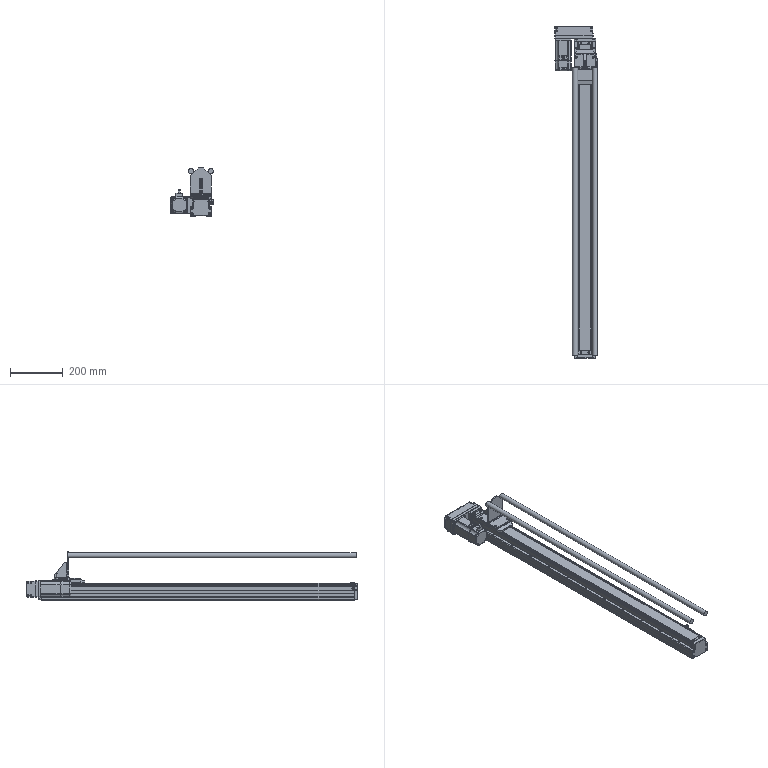Part | NX | features BREP 20, FILLET_WELD 5, FSET 5, DATUM_CSYS 3, EXTRUDE 3, MOVE_FACE 2, UNITE 2, CHAMFER 1, CYLINDER 1, SKETCH 1 | 55 solids | 2138 faces | box 163 x 1265 x 183 mm | volume 4732043 mm3 | plane 872 | cylinder 706 | cone 351 | torus 92 | spline 80 | sphere 37 | commonest cylinder face diameters 4 x75 5 x75 1 x51 2.5 x48 5.4 x48 0.4 x42